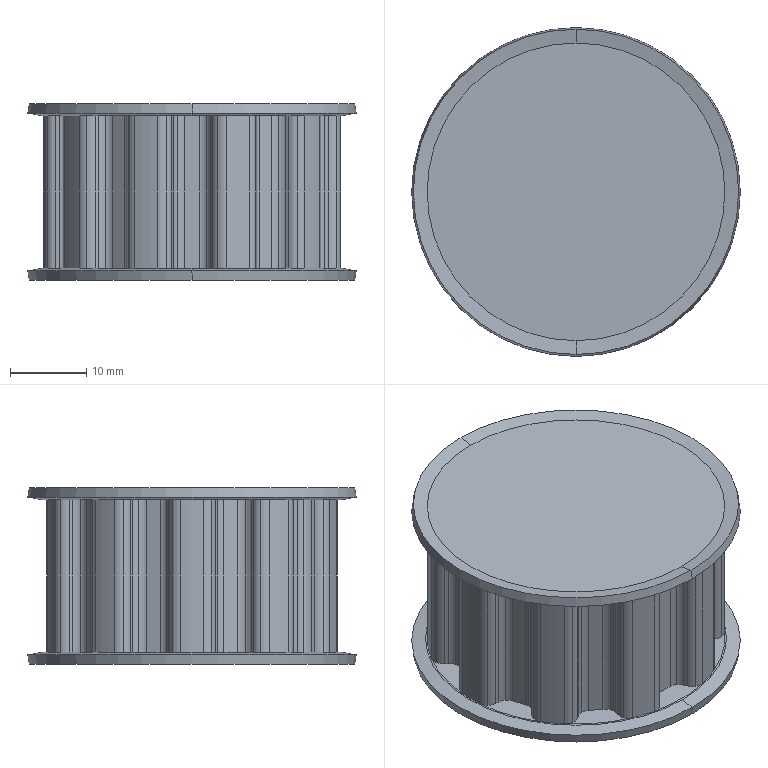Part | SolidWorks | features BaseBody 1 | 1 solid | 159 faces | box 43.118 x 43.118 x 23.179 mm | volume 24449 mm3 | cylinder 91 | plane 52 | cone 12 | torus 4 | commonest cylinder face diameters 3.2 x80 39.054 x11